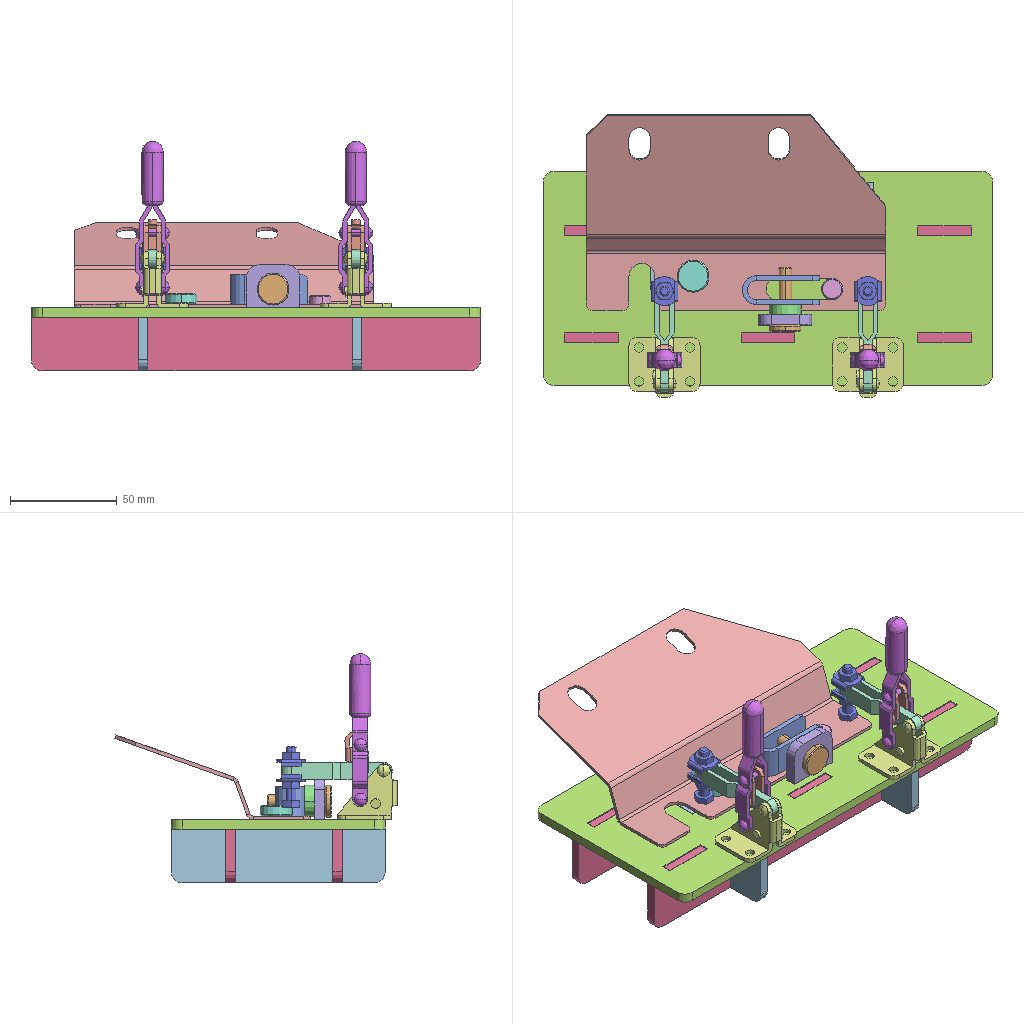Assembly | SolidWorks | 11 different items | 14 placed | box 210 x 132 x 107 mm
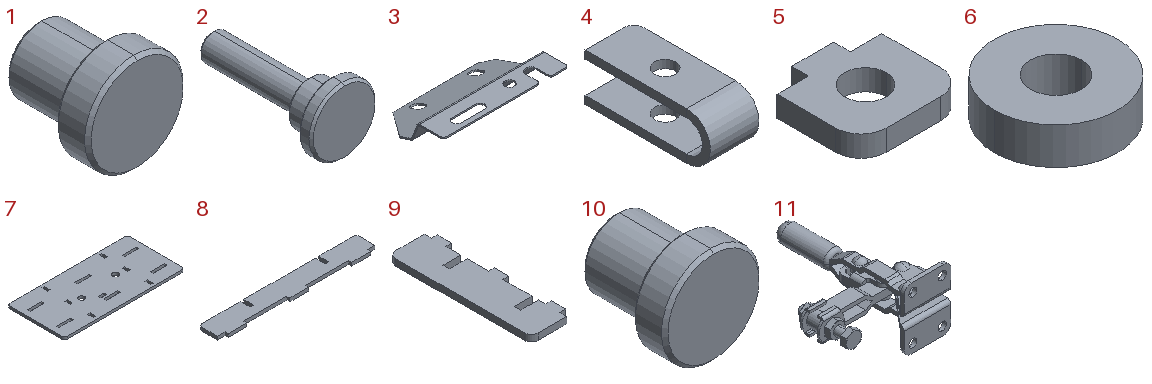Parts list (item | quantity | size | volume | features):
1 | x1 | 15 x 15 x 15 mm | 1654 mm3 | features Chamfer 1, Revolution 1
2 | x1 | 15 x 30 x 15 mm | 1548 mm3 | features Chamfer 1, Revolution 1
3 | x1 | 140 x 91.5 x 39.507 mm | 21022 mm3 | features ICE 2, Fillet 1, FlatPattern 1, SMBaseFlange 1, SheetMetal 1
4 | x1 | 14 x 36 x 13.6 mm | 2309 mm3 | features Fillet 1, FlatPattern 1, ICE 1, SMBaseFlange 1, SheetMetal 1
5 | x1 | 25 x 24 x 5 mm | 2230 mm3 | features FlatPattern 1, SMBaseFlange 1, SheetMetal 1
6 | x1 | 15 x 15 x 4.5 mm | 659.357 mm3 | features FlatPattern 1, SMBaseFlange 1, SheetMetal 1
7 | x1 | 210 x 100 x 4.5 mm | 89183 mm3 | features FlatPattern 1, SMBaseFlange 1, SheetMetal 1
8 | x2 | 210 x 29 x 4.5 mm | 24400 mm3 | features FlatPattern 1, SMBaseFlange 1, SheetMetal 1
9 | x2 | 29 x 100 x 4.5 mm | 11235 mm3 | features FlatPattern 1, SMBaseFlange 1, SheetMetal 1
10 | x1 | 15 x 15 x 15 mm | 1734 mm3 | features Chamfer 1, Revolution 1
11 | x2 | 56.45 x 77.62 x 33.3 mm | 10418 mm3 | features BaseBody 5
Mates (type | each side: item.copy, entity, surface, feature):
Coincident | 3.1 face plane Base-Flange1 | 4.1 face plane Base-Flange1
Coincident | 3.1 face plane Cut-Extrude2 | 4.1 face plane Base-Flange1
DistanceDim | 4.1 face cylinder Cut-Extrude1 | 3.1 face cylinder Cut-Extrude2
InPlace | 3.1 face plane Base-Flange1 | 7.1 plane
Concentric | 3.1 face cylinder Cut-Extrude2 | 1.1 face cylinder Revolve1
Concentric | 3.1 face cylinder Cut-Extrude2 | 10.1 face cylinder Revolve1
Coincident | 3.1 face plane Base-Flange1 | 10.1 face plane Revolve1
Concentric | 4.1 face cylinder Cut-Extrude1 | 2.1 face cylinder Revolve1
DistanceDim | 2.1 face plane Revolve1 | 4.1 face plane Base-Flange1
InPlace | 2.1 face plane Revolve1 | 5.1 plane
InPlace | 5.1 face plane Base-Flange1 | 6.1 plane
Coincident | 7.1 face plane Base-Flange1 | 1.1 face plane Revolve1
InPlace | 8.1 plane | assembly plane
InPlace | 9.1 plane | assembly plane
Coincident | 7.1 face plane Base-Flange1 | 11.1 face plane TC1-1 vertical flange-base toggle clamp[TCS1-1].step-1/_TCS1-1(seat).step-1-solid1
DistanceDim | 3.1 face plane Base-Flange1 | 11.1 face plane TC1-1 vertical flange-base toggle clamp[TCS1-1].step-1/_TCS1-1(bolt).step-1-solid1
DistanceDim | 11.1 face plane TC1-1 vertical flange-base toggle clamp[TCS1-1].step-1/_TCS1-1(seat).step-1-solid1 | 7.1 face plane Base-Flange1